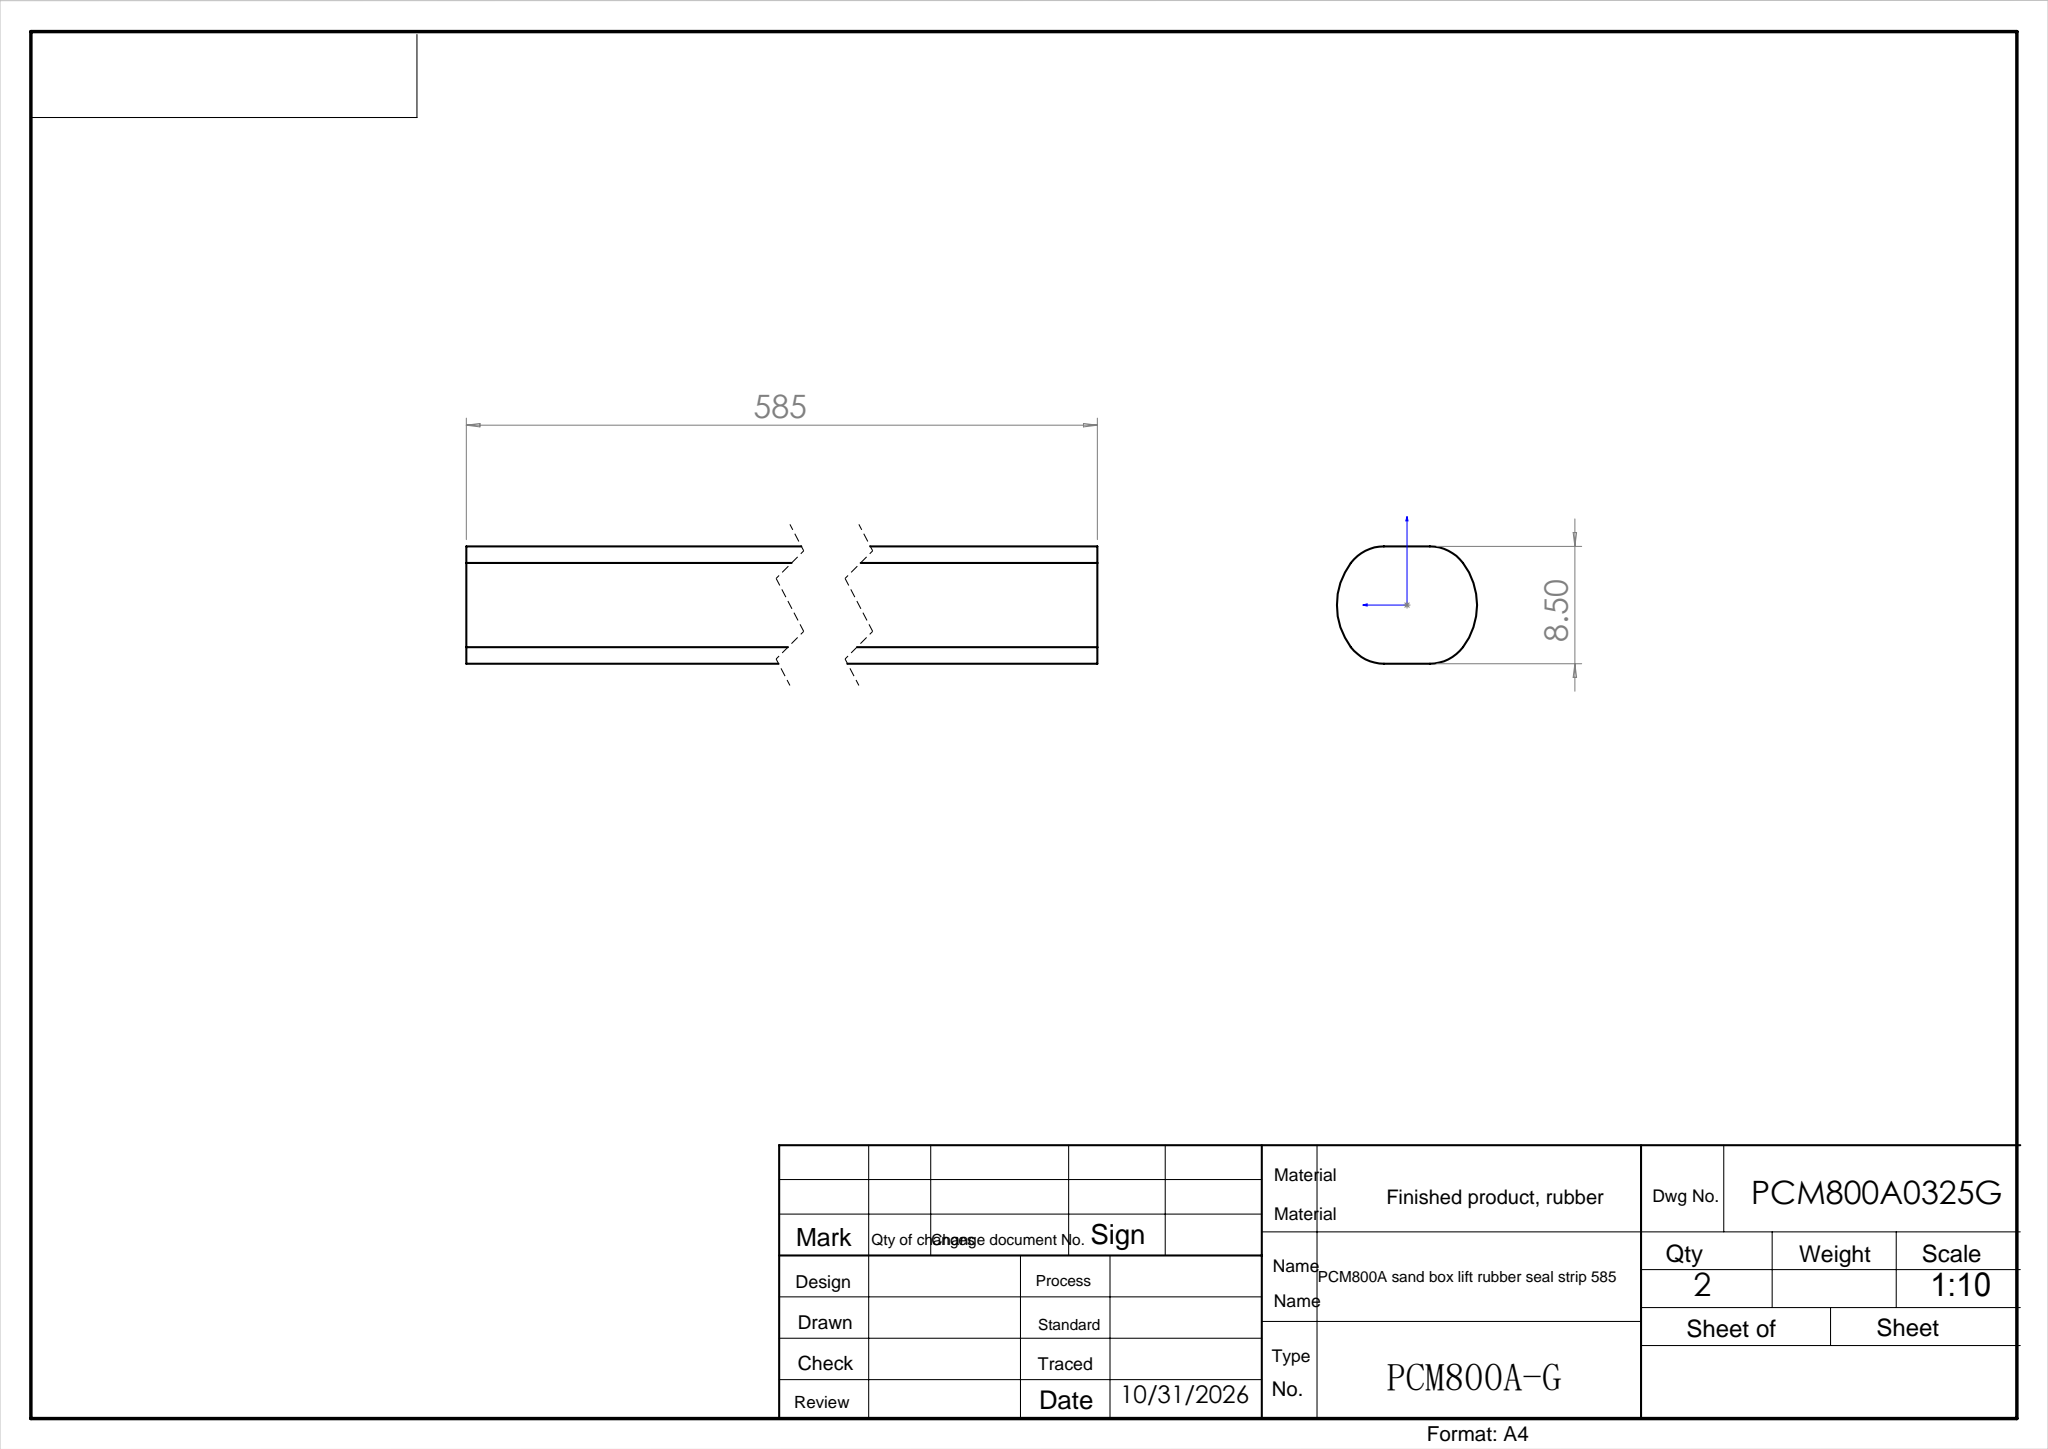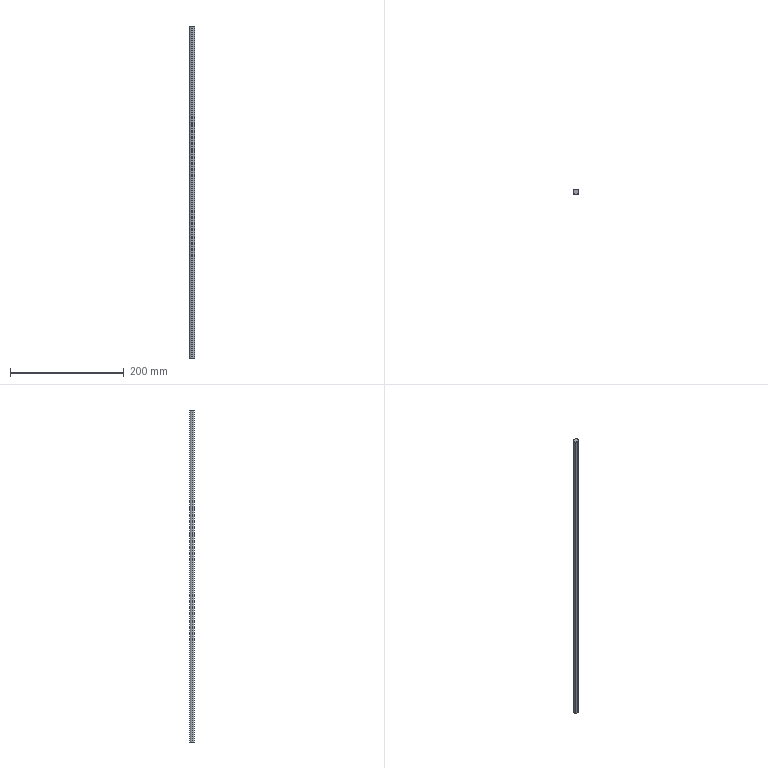Part | SolidWorks | features Extrusion 1 | 1 solid | 11 faces | box 10.158 x 8.5 x 585 mm | volume 43311 mm3 | cylinder 7 | plane 4 | commonest cylinder face diameters 6 x4 10.158 x3
STEP:
#1=CARTESIAN_POINT('',(-5.079,0.,585.));
#2=VERTEX_POINT('',#1);
#3=CARTESIAN_POINT('',(-4.059,-3.054,585.));
#4=VERTEX_POINT('',#3);
#5=CARTESIAN_POINT('',(0.,0.,585.));
#6=DIRECTION('',(0.,0.,1.));
#7=DIRECTION('',(1.,0.,0.));
#8=AXIS2_PLACEMENT_3D('',#5,#6,#7);
#9=CIRCLE('',#8,5.079);
#10=EDGE_CURVE('',#2,#4,#9,.T.);
#11=ORIENTED_EDGE('',*,*,#10,.F.);
#12=CARTESIAN_POINT('',(-5.079,0.,0.));
#13=VERTEX_POINT('',#12);
#14=CARTESIAN_POINT('',(-5.079,0.,585.));
#15=DIRECTION('',(0.,0.,-1.));
#16=VECTOR('',#15,1000.);
#17=LINE('',#14,#16);
#18=EDGE_CURVE('',#2,#13,#17,.T.);
#19=ORIENTED_EDGE('',*,*,#18,.T.);
#20=CARTESIAN_POINT('',(-4.059,-3.054,0.));
#21=VERTEX_POINT('',#20);
#22=CARTESIAN_POINT('',(0.,0.,0.));
#23=DIRECTION('',(0.,0.,1.));
#24=DIRECTION('',(1.,0.,0.));
#25=AXIS2_PLACEMENT_3D('',#22,#23,#24);
#26=CIRCLE('',#25,5.079);
#27=EDGE_CURVE('',#13,#21,#26,.T.);
#28=ORIENTED_EDGE('',*,*,#27,.T.);
#29=CARTESIAN_POINT('',(-4.059,-3.054,585.));
#30=DIRECTION('',(0.,0.,-1.));
#31=VECTOR('',#30,1000.);
#32=LINE('',#29,#31);
#33=EDGE_CURVE('',#4,#21,#32,.T.);
#34=ORIENTED_EDGE('',*,*,#33,.F.);
#35=EDGE_LOOP('',(#11,#19,#28,#34));
#36=FACE_OUTER_BOUND('',#35,.T.);
#37=CARTESIAN_POINT('',(0.,0.,585.));
#38=DIRECTION('',(0.,0.,-1.));
#39=DIRECTION('',(-1.,0.,0.));
#40=AXIS2_PLACEMENT_3D('',#37,#38,#39);
#41=CYLINDRICAL_SURFACE('',#40,5.079);
#42=ADVANCED_FACE('',(#36),#41,.T.);
#43=CARTESIAN_POINT('',(-1.661,4.25,0.));
#44=VERTEX_POINT('',#43);
#45=CARTESIAN_POINT('',(-4.059,3.054,0.));
#46=VERTEX_POINT('',#45);
#47=CARTESIAN_POINT('',(-1.661,1.25,0.));
#48=DIRECTION('',(0.,0.,1.));
#49=DIRECTION('',(-1.,0.,0.));
#50=AXIS2_PLACEMENT_3D('',#47,#48,#49);
#51=CIRCLE('',#50,3.);
#52=EDGE_CURVE('',#44,#46,#51,.T.);
#53=ORIENTED_EDGE('',*,*,#52,.T.);
#54=CARTESIAN_POINT('',(-4.059,3.054,585.));
#55=VERTEX_POINT('',#54);
#56=CARTESIAN_POINT('',(-4.059,3.054,585.));
#57=DIRECTION('',(0.,0.,-1.));
#58=VECTOR('',#57,1000.);
#59=LINE('',#56,#58);
#60=EDGE_CURVE('',#55,#46,#59,.T.);
#61=ORIENTED_EDGE('',*,*,#60,.F.);
#62=CARTESIAN_POINT('',(-1.661,4.25,585.));
#63=VERTEX_POINT('',#62);
#64=CARTESIAN_POINT('',(-1.661,1.25,585.));
#65=DIRECTION('',(0.,0.,1.));
#66=DIRECTION('',(-1.,0.,0.));
#67=AXIS2_PLACEMENT_3D('',#64,#65,#66);
#68=CIRCLE('',#67,3.);
#69=EDGE_CURVE('',#63,#55,#68,.T.);
#70=ORIENTED_EDGE('',*,*,#69,.F.);
#71=CARTESIAN_POINT('',(-1.661,4.25,585.));
#72=DIRECTION('',(0.,0.,-1.));
#73=VECTOR('',#72,1000.);
#74=LINE('',#71,#73);
#75=EDGE_CURVE('',#63,#44,#74,.T.);
#76=ORIENTED_EDGE('',*,*,#75,.T.);
#77=EDGE_LOOP('',(#53,#61,#70,#76));
#78=FACE_OUTER_BOUND('',#77,.T.);
#79=CARTESIAN_POINT('',(-1.661,1.25,585.));
#80=DIRECTION('',(0.,0.,-1.));
#81=DIRECTION('',(-1.,0.,0.));
#82=AXIS2_PLACEMENT_3D('',#79,#80,#81);
#83=CYLINDRICAL_SURFACE('',#82,3.);
#84=ADVANCED_FACE('',(#78),#83,.T.);
#85=ORIENTED_EDGE('',*,*,#18,.F.);
#86=CARTESIAN_POINT('',(0.,0.,585.));
#87=DIRECTION('',(0.,0.,1.));
#88=DIRECTION('',(1.,0.,0.));
#89=AXIS2_PLACEMENT_3D('',#86,#87,#88);
#90=CIRCLE('',#89,5.079);
#91=EDGE_CURVE('',#55,#2,#90,.T.);
#92=ORIENTED_EDGE('',*,*,#91,.F.);
#93=ORIENTED_EDGE('',*,*,#60,.T.);
#94=CARTESIAN_POINT('',(0.,0.,0.));
#95=DIRECTION('',(0.,0.,1.));
#96=DIRECTION('',(1.,0.,0.));
#97=AXIS2_PLACEMENT_3D('',#94,#95,#96);
#98=CIRCLE('',#97,5.079);
#99=EDGE_CURVE('',#46,#13,#98,.T.);
#100=ORIENTED_EDGE('',*,*,#99,.T.);
#101=EDGE_LOOP('',(#85,#92,#93,#100));
#102=FACE_OUTER_BOUND('',#101,.T.);
#103=CARTESIAN_POINT('',(0.,0.,585.));
#104=DIRECTION('',(0.,0.,-1.));
#105=DIRECTION('',(-1.,0.,0.));
#106=AXIS2_PLACEMENT_3D('',#103,#104,#105);
#107=CYLINDRICAL_SURFACE('',#106,5.079);
#108=ADVANCED_FACE('',(#102),#107,.T.);
#109=CARTESIAN_POINT('',(-1.661,-4.25,0.));
#110=VERTEX_POINT('',#109);
#111=CARTESIAN_POINT('',(-1.661,-1.25,0.));
#112=DIRECTION('',(0.,0.,1.));
#113=DIRECTION('',(1.,0.,0.));
#114=AXIS2_PLACEMENT_3D('',#111,#112,#113);
#115=CIRCLE('',#114,3.);
#116=EDGE_CURVE('',#21,#110,#115,.T.);
#117=ORIENTED_EDGE('',*,*,#116,.T.);
#118=CARTESIAN_POINT('',(-1.661,-4.25,585.));
#119=VERTEX_POINT('',#118);
#120=CARTESIAN_POINT('',(-1.661,-4.25,585.));
#121=DIRECTION('',(0.,0.,-1.));
#122=VECTOR('',#121,1000.);
#123=LINE('',#120,#122);
#124=EDGE_CURVE('',#119,#110,#123,.T.);
#125=ORIENTED_EDGE('',*,*,#124,.F.);
#126=CARTESIAN_POINT('',(-1.661,-1.25,585.));
#127=DIRECTION('',(0.,0.,1.));
#128=DIRECTION('',(1.,0.,0.));
#129=AXIS2_PLACEMENT_3D('',#126,#127,#128);
#130=CIRCLE('',#129,3.);
#131=EDGE_CURVE('',#4,#119,#130,.T.);
#132=ORIENTED_EDGE('',*,*,#131,.F.);
#133=ORIENTED_EDGE('',*,*,#33,.T.);
#134=EDGE_LOOP('',(#117,#125,#132,#133));
#135=FACE_OUTER_BOUND('',#134,.T.);
#136=CARTESIAN_POINT('',(-1.661,-1.25,585.));
#137=DIRECTION('',(0.,0.,-1.));
#138=DIRECTION('',(-1.,0.,0.));
#139=AXIS2_PLACEMENT_3D('',#136,#137,#138);
#140=CYLINDRICAL_SURFACE('',#139,3.);
#141=ADVANCED_FACE('',(#135),#140,.T.);
#142=CARTESIAN_POINT('',(1.661,-4.25,0.));
#143=VERTEX_POINT('',#142);
#144=CARTESIAN_POINT('',(-1.661,-4.25,0.));
#145=DIRECTION('',(1.,0.,0.));
#146=VECTOR('',#145,1000.);
#147=LINE('',#144,#146);
#148=EDGE_CURVE('',#110,#143,#147,.T.);
#149=ORIENTED_EDGE('',*,*,#148,.T.);
#150=CARTESIAN_POINT('',(1.661,-4.25,585.));
#151=VERTEX_POINT('',#150);
#152=CARTESIAN_POINT('',(1.661,-4.25,585.));
#153=DIRECTION('',(0.,0.,-1.));
#154=VECTOR('',#153,1000.);
#155=LINE('',#152,#154);
#156=EDGE_CURVE('',#151,#143,#155,.T.);
#157=ORIENTED_EDGE('',*,*,#156,.F.);
#158=CARTESIAN_POINT('',(-1.661,-4.25,585.));
#159=DIRECTION('',(1.,0.,0.));
#160=VECTOR('',#159,1000.);
#161=LINE('',#158,#160);
#162=EDGE_CURVE('',#119,#151,#161,.T.);
#163=ORIENTED_EDGE('',*,*,#162,.F.);
#164=ORIENTED_EDGE('',*,*,#124,.T.);
#165=EDGE_LOOP('',(#149,#157,#163,#164));
#166=FACE_OUTER_BOUND('',#165,.T.);
#167=CARTESIAN_POINT('',(-1.661,-4.25,585.));
#168=DIRECTION('',(0.,1.,0.));
#169=DIRECTION('',(0.,0.,1.));
#170=AXIS2_PLACEMENT_3D('',#167,#168,#169);
#171=PLANE('',#170);
#172=ADVANCED_FACE('',(#166),#171,.F.);
#173=CARTESIAN_POINT('',(4.059,-3.054,0.));
#174=VERTEX_POINT('',#173);
#175=CARTESIAN_POINT('',(1.661,-1.25,0.));
#176=DIRECTION('',(0.,0.,1.));
#177=DIRECTION('',(1.,0.,0.));
#178=AXIS2_PLACEMENT_3D('',#175,#176,#177);
#179=CIRCLE('',#178,3.);
#180=EDGE_CURVE('',#143,#174,#179,.T.);
#181=ORIENTED_EDGE('',*,*,#180,.T.);
#182=CARTESIAN_POINT('',(4.059,-3.054,585.));
#183=VERTEX_POINT('',#182);
#184=CARTESIAN_POINT('',(4.059,-3.054,585.));
#185=DIRECTION('',(0.,0.,-1.));
#186=VECTOR('',#185,1000.);
#187=LINE('',#184,#186);
#188=EDGE_CURVE('',#183,#174,#187,.T.);
#189=ORIENTED_EDGE('',*,*,#188,.F.);
#190=CARTESIAN_POINT('',(1.661,-1.25,585.));
#191=DIRECTION('',(0.,0.,1.));
#192=DIRECTION('',(1.,0.,0.));
#193=AXIS2_PLACEMENT_3D('',#190,#191,#192);
#194=CIRCLE('',#193,3.);
#195=EDGE_CURVE('',#151,#183,#194,.T.);
#196=ORIENTED_EDGE('',*,*,#195,.F.);
#197=ORIENTED_EDGE('',*,*,#156,.T.);
#198=EDGE_LOOP('',(#181,#189,#196,#197));
#199=FACE_OUTER_BOUND('',#198,.T.);
#200=CARTESIAN_POINT('',(1.661,-1.25,585.));
#201=DIRECTION('',(0.,0.,-1.));
#202=DIRECTION('',(-1.,0.,0.));
#203=AXIS2_PLACEMENT_3D('',#200,#201,#202);
#204=CYLINDRICAL_SURFACE('',#203,3.);
#205=ADVANCED_FACE('',(#199),#204,.T.);
#206=CARTESIAN_POINT('',(4.059,3.054,0.));
#207=VERTEX_POINT('',#206);
#208=CARTESIAN_POINT('',(0.,0.,0.));
#209=DIRECTION('',(0.,0.,1.));
#210=DIRECTION('',(1.,0.,0.));
#211=AXIS2_PLACEMENT_3D('',#208,#209,#210);
#212=CIRCLE('',#211,5.079);
#213=EDGE_CURVE('',#174,#207,#212,.T.);
#214=ORIENTED_EDGE('',*,*,#213,.T.);
#215=CARTESIAN_POINT('',(4.059,3.054,585.));
#216=VERTEX_POINT('',#215);
#217=CARTESIAN_POINT('',(4.059,3.054,585.));
#218=DIRECTION('',(0.,0.,-1.));
#219=VECTOR('',#218,1000.);
#220=LINE('',#217,#219);
#221=EDGE_CURVE('',#216,#207,#220,.T.);
#222=ORIENTED_EDGE('',*,*,#221,.F.);
#223=CARTESIAN_POINT('',(0.,0.,585.));
#224=DIRECTION('',(0.,0.,1.));
#225=DIRECTION('',(1.,0.,0.));
#226=AXIS2_PLACEMENT_3D('',#223,#224,#225);
#227=CIRCLE('',#226,5.079);
#228=EDGE_CURVE('',#183,#216,#227,.T.);
#229=ORIENTED_EDGE('',*,*,#228,.F.);
#230=ORIENTED_EDGE('',*,*,#188,.T.);
#231=EDGE_LOOP('',(#214,#222,#229,#230));
#232=FACE_OUTER_BOUND('',#231,.T.);
#233=CARTESIAN_POINT('',(0.,0.,585.));
#234=DIRECTION('',(0.,0.,-1.));
#235=DIRECTION('',(-1.,0.,0.));
#236=AXIS2_PLACEMENT_3D('',#233,#234,#235);
#237=CYLINDRICAL_SURFACE('',#236,5.079);
#238=ADVANCED_FACE('',(#232),#237,.T.);
#239=CARTESIAN_POINT('',(1.661,4.25,0.));
#240=VERTEX_POINT('',#239);
#241=CARTESIAN_POINT('',(1.661,1.25,0.));
#242=DIRECTION('',(0.,0.,1.));
#243=DIRECTION('',(1.,0.,0.));
#244=AXIS2_PLACEMENT_3D('',#241,#242,#243);
#245=CIRCLE('',#244,3.);
#246=EDGE_CURVE('',#207,#240,#245,.T.);
#247=ORIENTED_EDGE('',*,*,#246,.T.);
#248=CARTESIAN_POINT('',(1.661,4.25,585.));
#249=VERTEX_POINT('',#248);
#250=CARTESIAN_POINT('',(1.661,4.25,585.));
#251=DIRECTION('',(0.,0.,-1.));
#252=VECTOR('',#251,1000.);
#253=LINE('',#250,#252);
#254=EDGE_CURVE('',#249,#240,#253,.T.);
#255=ORIENTED_EDGE('',*,*,#254,.F.);
#256=CARTESIAN_POINT('',(1.661,1.25,585.));
#257=DIRECTION('',(0.,0.,1.));
#258=DIRECTION('',(1.,0.,0.));
#259=AXIS2_PLACEMENT_3D('',#256,#257,#258);
#260=CIRCLE('',#259,3.);
#261=EDGE_CURVE('',#216,#249,#260,.T.);
#262=ORIENTED_EDGE('',*,*,#261,.F.);
#263=ORIENTED_EDGE('',*,*,#221,.T.);
#264=EDGE_LOOP('',(#247,#255,#262,#263));
#265=FACE_OUTER_BOUND('',#264,.T.);
#266=CARTESIAN_POINT('',(1.661,1.25,585.));
#267=DIRECTION('',(0.,0.,-1.));
#268=DIRECTION('',(-1.,0.,0.));
#269=AXIS2_PLACEMENT_3D('',#266,#267,#268);
#270=CYLINDRICAL_SURFACE('',#269,3.);
#271=ADVANCED_FACE('',(#265),#270,.T.);
#272=CARTESIAN_POINT('',(-1.661,4.25,0.));
#273=DIRECTION('',(-1.,0.,0.));
#274=VECTOR('',#273,1000.);
#275=LINE('',#272,#274);
#276=EDGE_CURVE('',#240,#44,#275,.T.);
#277=ORIENTED_EDGE('',*,*,#276,.T.);
#278=ORIENTED_EDGE('',*,*,#75,.F.);
#279=CARTESIAN_POINT('',(-1.661,4.25,585.));
#280=DIRECTION('',(-1.,0.,0.));
#281=VECTOR('',#280,1000.);
#282=LINE('',#279,#281);
#283=EDGE_CURVE('',#249,#63,#282,.T.);
#284=ORIENTED_EDGE('',*,*,#283,.F.);
#285=ORIENTED_EDGE('',*,*,#254,.T.);
#286=EDGE_LOOP('',(#277,#278,#284,#285));
#287=FACE_OUTER_BOUND('',#286,.T.);
#288=CARTESIAN_POINT('',(-1.661,4.25,585.));
#289=DIRECTION('',(0.,-1.,0.));
#290=DIRECTION('',(0.,0.,-1.));
#291=AXIS2_PLACEMENT_3D('',#288,#289,#290);
#292=PLANE('',#291);
#293=ADVANCED_FACE('',(#287),#292,.F.);
#294=ORIENTED_EDGE('',*,*,#69,.T.);
#295=ORIENTED_EDGE('',*,*,#91,.T.);
#296=ORIENTED_EDGE('',*,*,#10,.T.);
#297=ORIENTED_EDGE('',*,*,#131,.T.);
#298=ORIENTED_EDGE('',*,*,#162,.T.);
#299=ORIENTED_EDGE('',*,*,#195,.T.);
#300=ORIENTED_EDGE('',*,*,#228,.T.);
#301=ORIENTED_EDGE('',*,*,#261,.T.);
#302=ORIENTED_EDGE('',*,*,#283,.T.);
#303=EDGE_LOOP('',(#294,#295,#296,#297,#298,#299,#300,#301,#302));
#304=FACE_OUTER_BOUND('',#303,.T.);
#305=CARTESIAN_POINT('',(-1.661,1.25,585.));
#306=DIRECTION('',(0.,0.,-1.));
#307=DIRECTION('',(-1.,0.,0.));
#308=AXIS2_PLACEMENT_3D('',#305,#306,#307);
#309=PLANE('',#308);
#310=ADVANCED_FACE('',(#304),#309,.F.);
#311=ORIENTED_EDGE('',*,*,#52,.F.);
#312=ORIENTED_EDGE('',*,*,#276,.F.);
#313=ORIENTED_EDGE('',*,*,#246,.F.);
#314=ORIENTED_EDGE('',*,*,#213,.F.);
#315=ORIENTED_EDGE('',*,*,#180,.F.);
#316=ORIENTED_EDGE('',*,*,#148,.F.);
#317=ORIENTED_EDGE('',*,*,#116,.F.);
#318=ORIENTED_EDGE('',*,*,#27,.F.);
#319=ORIENTED_EDGE('',*,*,#99,.F.);
#320=EDGE_LOOP('',(#311,#312,#313,#314,#315,#316,#317,#318,#319));
#321=FACE_OUTER_BOUND('',#320,.T.);
#322=CARTESIAN_POINT('',(-1.661,1.25,0.));
#323=DIRECTION('',(0.,0.,-1.));
#324=DIRECTION('',(-1.,0.,0.));
#325=AXIS2_PLACEMENT_3D('',#322,#323,#324);
#326=PLANE('',#325);
#327=ADVANCED_FACE('',(#321),#326,.T.);
#328=CLOSED_SHELL('',(#42,#84,#108,#141,#172,#205,#238,#271,#293,#310,#327));
#329=MANIFOLD_SOLID_BREP('',#328);
#330=CARTESIAN_POINT('',(0.,0.,0.));
#331=DIRECTION('',(0.,0.,1.));
#332=DIRECTION('',(1.,0.,0.));
#333=AXIS2_PLACEMENT_3D('',#330,#331,#332);
#334=(LENGTH_UNIT()NAMED_UNIT(*)SI_UNIT(.MILLI.,.METRE.));
#335=UNCERTAINTY_MEASURE_WITH_UNIT(LENGTH_MEASURE(0.00001),#334,'','');
#336=(NAMED_UNIT(*)PLANE_ANGLE_UNIT()SI_UNIT($,.RADIAN.));
#337=(NAMED_UNIT(*)SI_UNIT($,.STERADIAN.)SOLID_ANGLE_UNIT());
#338=(GEOMETRIC_REPRESENTATION_CONTEXT(3)GLOBAL_UNCERTAINTY_ASSIGNED_CONTEXT((#335))GLOBAL_UNIT_ASSIGNED_CONTEXT((#334,#336,#337))REPRESENTATION_CONTEXT('',''));
#339=ADVANCED_BREP_SHAPE_REPRESENTATION('',(#329,#333),#338);